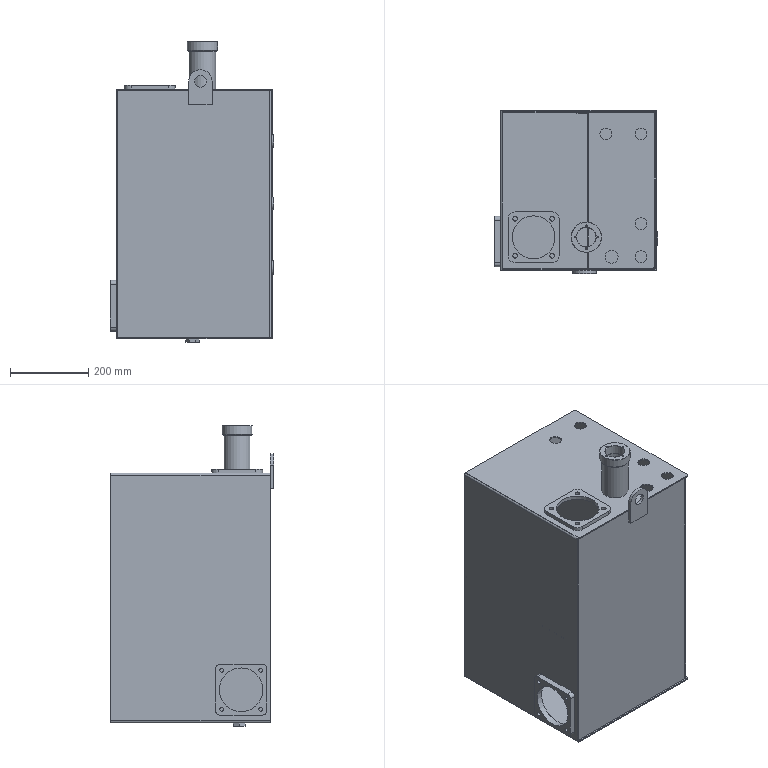Part | STEP file | COMPOUND | 15 solids | 226 faces | box 419 x 418 x 771 mm | volume 5464093 mm3 | plane 112 | cylinder 98 | cone 15 | torus 1 | commonest cylinder face diameters 10 x25 4 x11 6 x9 8 x7 30 x7 20 x6